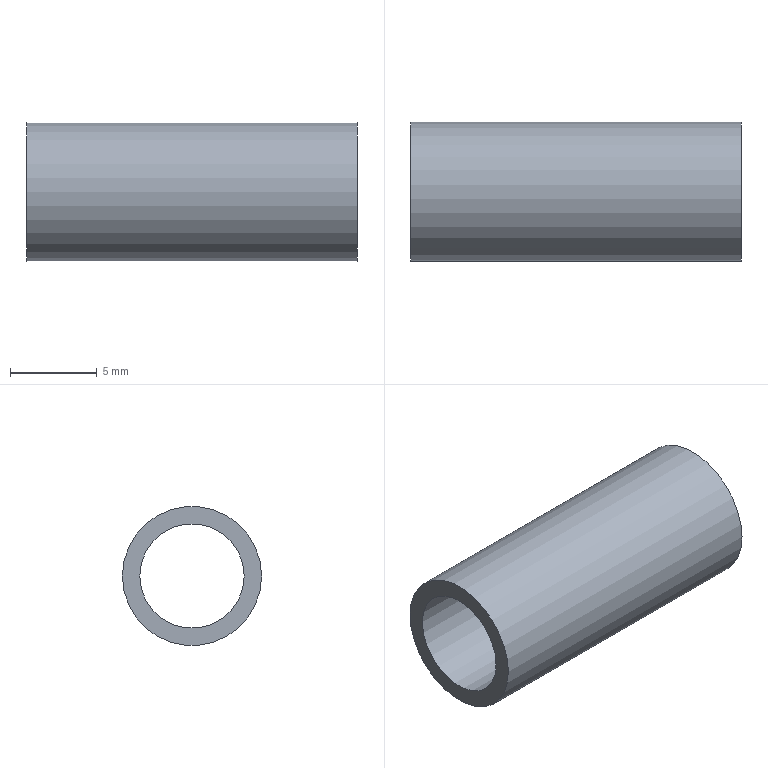Part | STEP file | 1-43.14 | 1 solid | 4 faces | box 19 x 8 x 8 mm | volume 417.832 mm3 | plane 2 | cylinder 2 | commonest cylinder face diameters 6 x1 8 x1
STEP:
#1=CARTESIAN_POINT('',(0.,0.,0.));
#2=DIRECTION('',(0.,0.,1.));
#3=DIRECTION('',(1.,0.,0.));
#4=AXIS2_PLACEMENT_3D('',#1,#2,#3);
#5=CARTESIAN_POINT('',(9.5,4.,0.));
#6=VERTEX_POINT('',#5);
#7=CARTESIAN_POINT('',(9.5,0.,0.));
#8=DIRECTION('',(1.,0.,0.));
#9=DIRECTION('',(0.,1.,0.));
#10=AXIS2_PLACEMENT_3D('',#7,#8,#9);
#11=CIRCLE('',#10,4.);
#12=CARTESIAN_POINT('',(9.5,-1.072,0.));
#13=DIRECTION('',(1.,0.,0.));
#14=DIRECTION('',(0.,1.,0.));
#15=AXIS2_PLACEMENT_3D('',#12,#13,#14);
#16=PLANE('',#15);
#17=CARTESIAN_POINT('',(1.072,0.));
#18=DIRECTION('',(1.,0.));
#19=AXIS2_PLACEMENT_2D('',#17,#18);
#20=CIRCLE('',#19,4.);
#21=(GEOMETRIC_REPRESENTATION_CONTEXT(2)PARAMETRIC_REPRESENTATION_CONTEXT()REPRESENTATION_CONTEXT('',''));
#22=DEFINITIONAL_REPRESENTATION('',(#20),#21);
#23=PCURVE('',#16,#22);
#24=CARTESIAN_POINT('',(9.5,0.,0.));
#25=DIRECTION('',(-1.,0.,0.));
#26=DIRECTION('',(0.,1.,0.));
#27=AXIS2_PLACEMENT_3D('',#24,#25,#26);
#28=CYLINDRICAL_SURFACE('',#27,4.);
#29=CARTESIAN_POINT('',(6.283,0.));
#30=DIRECTION('',(-1.,0.));
#31=VECTOR('',#30,1.);
#32=LINE('',#29,#31);
#33=(GEOMETRIC_REPRESENTATION_CONTEXT(2)PARAMETRIC_REPRESENTATION_CONTEXT()REPRESENTATION_CONTEXT('',''));
#34=DEFINITIONAL_REPRESENTATION('',(#32),#33);
#35=PCURVE('',#28,#34);
#36=SURFACE_CURVE('',#11,(#23,#35),.PCURVE_S1.);
#37=EDGE_CURVE('',#6,#6,#36,.T.);
#38=ORIENTED_EDGE('',*,*,#37,.T.);
#39=EDGE_LOOP('',(#38));
#40=FACE_BOUND('',#39,.T.);
#41=CARTESIAN_POINT('',(9.5,3.,0.));
#42=VERTEX_POINT('',#41);
#43=CARTESIAN_POINT('',(9.5,0.,0.));
#44=DIRECTION('',(-1.,0.,0.));
#45=DIRECTION('',(0.,1.,0.));
#46=AXIS2_PLACEMENT_3D('',#43,#44,#45);
#47=CIRCLE('',#46,3.);
#48=CARTESIAN_POINT('',(4.072,0.));
#49=CARTESIAN_POINT('',(4.072,-5.196));
#50=CARTESIAN_POINT('',(-0.4282,-2.598));
#51=CARTESIAN_POINT('',(-4.928,0.));
#52=CARTESIAN_POINT('',(-0.4282,2.598));
#53=CARTESIAN_POINT('',(4.072,5.196));
#54=CARTESIAN_POINT('',(4.072,0.));
#55=(BOUNDED_CURVE()B_SPLINE_CURVE(2,(#48,#49,#50,#51,#52,#53,#54),.UNSPECIFIED.,.T.,.F.)B_SPLINE_CURVE_WITH_KNOTS((1,2,2,2,2,1),(-2.094,0.,2.094,4.189,6.283,8.378),.UNSPECIFIED.)CURVE()GEOMETRIC_REPRESENTATION_ITEM()RATIONAL_B_SPLINE_CURVE((1.,0.5,1.,0.5,1.,0.5,1.))REPRESENTATION_ITEM(''));
#56=(GEOMETRIC_REPRESENTATION_CONTEXT(2)PARAMETRIC_REPRESENTATION_CONTEXT()REPRESENTATION_CONTEXT('',''));
#57=DEFINITIONAL_REPRESENTATION('',(#55),#56);
#58=PCURVE('',#16,#57);
#59=CARTESIAN_POINT('',(9.5,0.,0.));
#60=DIRECTION('',(-1.,0.,0.));
#61=DIRECTION('',(0.,1.,0.));
#62=AXIS2_PLACEMENT_3D('',#59,#60,#61);
#63=CYLINDRICAL_SURFACE('',#62,3.);
#64=CARTESIAN_POINT('',(0.,0.));
#65=DIRECTION('',(1.,0.));
#66=VECTOR('',#65,1.);
#67=LINE('',#64,#66);
#68=(GEOMETRIC_REPRESENTATION_CONTEXT(2)PARAMETRIC_REPRESENTATION_CONTEXT()REPRESENTATION_CONTEXT('',''));
#69=DEFINITIONAL_REPRESENTATION('',(#67),#68);
#70=PCURVE('',#63,#69);
#71=SURFACE_CURVE('',#47,(#58,#70),.PCURVE_S1.);
#72=EDGE_CURVE('',#42,#42,#71,.T.);
#73=ORIENTED_EDGE('',*,*,#72,.T.);
#74=EDGE_LOOP('',(#73));
#75=FACE_BOUND('',#74,.T.);
#76=ADVANCED_FACE('',(#40,#75),#16,.T.);
#77=CARTESIAN_POINT('',(-9.5,4.,0.));
#78=VERTEX_POINT('',#77);
#79=CARTESIAN_POINT('',(-9.5,0.,0.));
#80=DIRECTION('',(1.,0.,0.));
#81=DIRECTION('',(0.,1.,0.));
#82=AXIS2_PLACEMENT_3D('',#79,#80,#81);
#83=CIRCLE('',#82,4.);
#84=CARTESIAN_POINT('',(-9.5,-1.072,0.));
#85=DIRECTION('',(1.,0.,0.));
#86=DIRECTION('',(0.,1.,0.));
#87=AXIS2_PLACEMENT_3D('',#84,#85,#86);
#88=PLANE('',#87);
#89=CARTESIAN_POINT('',(1.072,0.));
#90=DIRECTION('',(1.,0.));
#91=AXIS2_PLACEMENT_2D('',#89,#90);
#92=CIRCLE('',#91,4.);
#93=(GEOMETRIC_REPRESENTATION_CONTEXT(2)PARAMETRIC_REPRESENTATION_CONTEXT()REPRESENTATION_CONTEXT('',''));
#94=DEFINITIONAL_REPRESENTATION('',(#92),#93);
#95=PCURVE('',#88,#94);
#96=CARTESIAN_POINT('',(6.283,19.));
#97=DIRECTION('',(-1.,0.));
#98=VECTOR('',#97,1.);
#99=LINE('',#96,#98);
#100=(GEOMETRIC_REPRESENTATION_CONTEXT(2)PARAMETRIC_REPRESENTATION_CONTEXT()REPRESENTATION_CONTEXT('',''));
#101=DEFINITIONAL_REPRESENTATION('',(#99),#100);
#102=PCURVE('',#28,#101);
#103=SURFACE_CURVE('',#83,(#95,#102),.PCURVE_S1.);
#104=EDGE_CURVE('',#78,#78,#103,.T.);
#105=ORIENTED_EDGE('',*,*,#104,.T.);
#106=EDGE_LOOP('',(#105));
#107=FACE_BOUND('',#106,.F.);
#108=CARTESIAN_POINT('',(-9.5,3.,0.));
#109=VERTEX_POINT('',#108);
#110=CARTESIAN_POINT('',(-9.5,0.,0.));
#111=DIRECTION('',(-1.,0.,0.));
#112=DIRECTION('',(0.,1.,0.));
#113=AXIS2_PLACEMENT_3D('',#110,#111,#112);
#114=CIRCLE('',#113,3.);
#115=CARTESIAN_POINT('',(4.072,0.));
#116=CARTESIAN_POINT('',(4.072,-5.196));
#117=CARTESIAN_POINT('',(-0.4282,-2.598));
#118=CARTESIAN_POINT('',(-4.928,0.));
#119=CARTESIAN_POINT('',(-0.4282,2.598));
#120=CARTESIAN_POINT('',(4.072,5.196));
#121=CARTESIAN_POINT('',(4.072,0.));
#122=(BOUNDED_CURVE()B_SPLINE_CURVE(2,(#115,#116,#117,#118,#119,#120,#121),.UNSPECIFIED.,.T.,.F.)B_SPLINE_CURVE_WITH_KNOTS((1,2,2,2,2,1),(-2.094,0.,2.094,4.189,6.283,8.378),.UNSPECIFIED.)CURVE()GEOMETRIC_REPRESENTATION_ITEM()RATIONAL_B_SPLINE_CURVE((1.,0.5,1.,0.5,1.,0.5,1.))REPRESENTATION_ITEM(''));
#123=(GEOMETRIC_REPRESENTATION_CONTEXT(2)PARAMETRIC_REPRESENTATION_CONTEXT()REPRESENTATION_CONTEXT('',''));
#124=DEFINITIONAL_REPRESENTATION('',(#122),#123);
#125=PCURVE('',#88,#124);
#126=CARTESIAN_POINT('',(0.,19.));
#127=DIRECTION('',(1.,0.));
#128=VECTOR('',#127,1.);
#129=LINE('',#126,#128);
#130=(GEOMETRIC_REPRESENTATION_CONTEXT(2)PARAMETRIC_REPRESENTATION_CONTEXT()REPRESENTATION_CONTEXT('',''));
#131=DEFINITIONAL_REPRESENTATION('',(#129),#130);
#132=PCURVE('',#63,#131);
#133=SURFACE_CURVE('',#114,(#125,#132),.PCURVE_S1.);
#134=EDGE_CURVE('',#109,#109,#133,.T.);
#135=ORIENTED_EDGE('',*,*,#134,.T.);
#136=EDGE_LOOP('',(#135));
#137=FACE_BOUND('',#136,.F.);
#138=ADVANCED_FACE('',(#107,#137),#88,.F.);
#139=CARTESIAN_POINT('',(9.5,4.,0.));
#140=DIRECTION('',(-1.,0.,0.));
#141=VECTOR('',#140,1.);
#142=LINE('',#139,#141);
#143=CARTESIAN_POINT('',(6.283,0.));
#144=DIRECTION('',(0.,1.));
#145=VECTOR('',#144,1.);
#146=LINE('',#143,#145);
#147=(GEOMETRIC_REPRESENTATION_CONTEXT(2)PARAMETRIC_REPRESENTATION_CONTEXT()REPRESENTATION_CONTEXT('',''));
#148=DEFINITIONAL_REPRESENTATION('',(#146),#147);
#149=PCURVE('',#28,#148);
#150=CARTESIAN_POINT('',(0.,0.));
#151=DIRECTION('',(0.,1.));
#152=VECTOR('',#151,1.);
#153=LINE('',#150,#152);
#154=(GEOMETRIC_REPRESENTATION_CONTEXT(2)PARAMETRIC_REPRESENTATION_CONTEXT()REPRESENTATION_CONTEXT('',''));
#155=DEFINITIONAL_REPRESENTATION('',(#153),#154);
#156=PCURVE('',#28,#155);
#157=SEAM_CURVE('',#142,(#149,#156),.PCURVE_S1.);
#158=EDGE_CURVE('',#6,#78,#157,.T.);
#159=ORIENTED_EDGE('',*,*,#158,.T.);
#160=ORIENTED_EDGE('',*,*,#104,.T.);
#161=ORIENTED_EDGE('',*,*,#158,.F.);
#162=ORIENTED_EDGE('',*,*,#37,.F.);
#163=EDGE_LOOP('',(#159,#160,#161,#162));
#164=FACE_BOUND('',#163,.T.);
#165=ADVANCED_FACE('',(#164),#28,.T.);
#166=ORIENTED_EDGE('',*,*,#72,.T.);
#167=CARTESIAN_POINT('',(9.5,3.,0.));
#168=DIRECTION('',(-1.,0.,0.));
#169=VECTOR('',#168,1.);
#170=LINE('',#167,#169);
#171=CARTESIAN_POINT('',(6.283,0.));
#172=DIRECTION('',(0.,1.));
#173=VECTOR('',#172,1.);
#174=LINE('',#171,#173);
#175=(GEOMETRIC_REPRESENTATION_CONTEXT(2)PARAMETRIC_REPRESENTATION_CONTEXT()REPRESENTATION_CONTEXT('',''));
#176=DEFINITIONAL_REPRESENTATION('',(#174),#175);
#177=PCURVE('',#63,#176);
#178=CARTESIAN_POINT('',(0.,0.));
#179=DIRECTION('',(0.,1.));
#180=VECTOR('',#179,1.);
#181=LINE('',#178,#180);
#182=(GEOMETRIC_REPRESENTATION_CONTEXT(2)PARAMETRIC_REPRESENTATION_CONTEXT()REPRESENTATION_CONTEXT('',''));
#183=DEFINITIONAL_REPRESENTATION('',(#181),#182);
#184=PCURVE('',#63,#183);
#185=SEAM_CURVE('',#170,(#177,#184),.PCURVE_S1.);
#186=EDGE_CURVE('',#42,#109,#185,.T.);
#187=ORIENTED_EDGE('',*,*,#186,.T.);
#188=ORIENTED_EDGE('',*,*,#134,.F.);
#189=ORIENTED_EDGE('',*,*,#186,.F.);
#190=EDGE_LOOP('',(#166,#187,#188,#189));
#191=FACE_BOUND('',#190,.F.);
#192=ADVANCED_FACE('',(#191),#63,.F.);
#193=CLOSED_SHELL('',(#76,#138,#165,#192));
#194=MANIFOLD_SOLID_BREP('',#193);
#195=(LENGTH_UNIT()NAMED_UNIT(*)SI_UNIT(.MILLI.,.METRE.));
#196=UNCERTAINTY_MEASURE_WITH_UNIT(LENGTH_MEASURE(0.0000001),#195,'','');
#197=(NAMED_UNIT(*)PLANE_ANGLE_UNIT()SI_UNIT($,.RADIAN.));
#198=(NAMED_UNIT(*)SI_UNIT($,.STERADIAN.)SOLID_ANGLE_UNIT());
#199=(GEOMETRIC_REPRESENTATION_CONTEXT(3)GLOBAL_UNCERTAINTY_ASSIGNED_CONTEXT((#196))GLOBAL_UNIT_ASSIGNED_CONTEXT((#195,#197,#198))REPRESENTATION_CONTEXT('',''));
#200=ADVANCED_BREP_SHAPE_REPRESENTATION('',(#4,#194),#199);